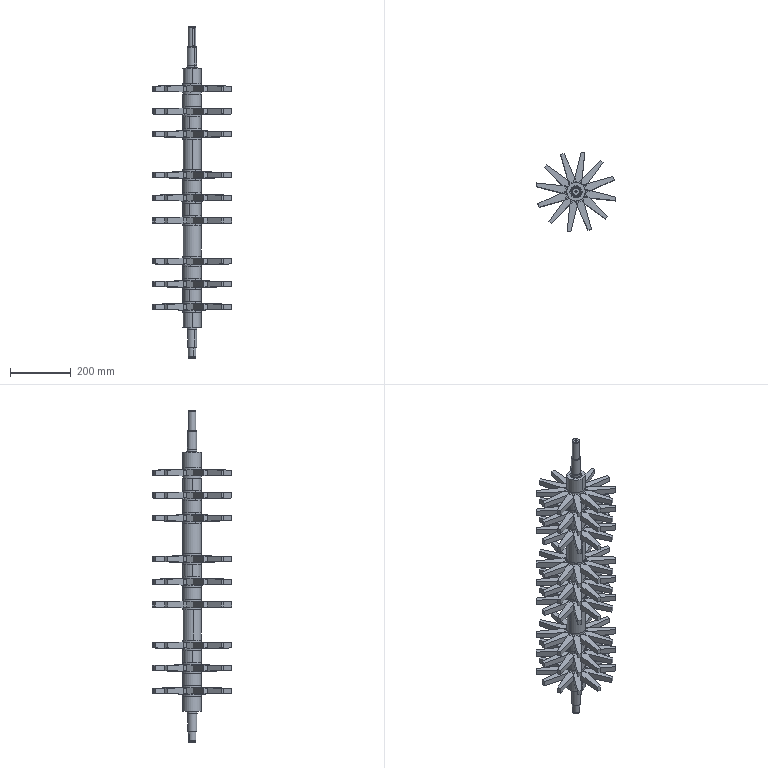Part | SolidWorks | features LayoutProfileFeature 1 | 27 solids | 1709 faces | box 262.006 x 262.006 x 1096 mm | volume 5906845 mm3 | plane 1529 | cylinder 136 | cone 36 | spline 8 | commonest cylinder face diameters 62 x36 40 x20 60 x20 15 x18 9 x12 25 x8